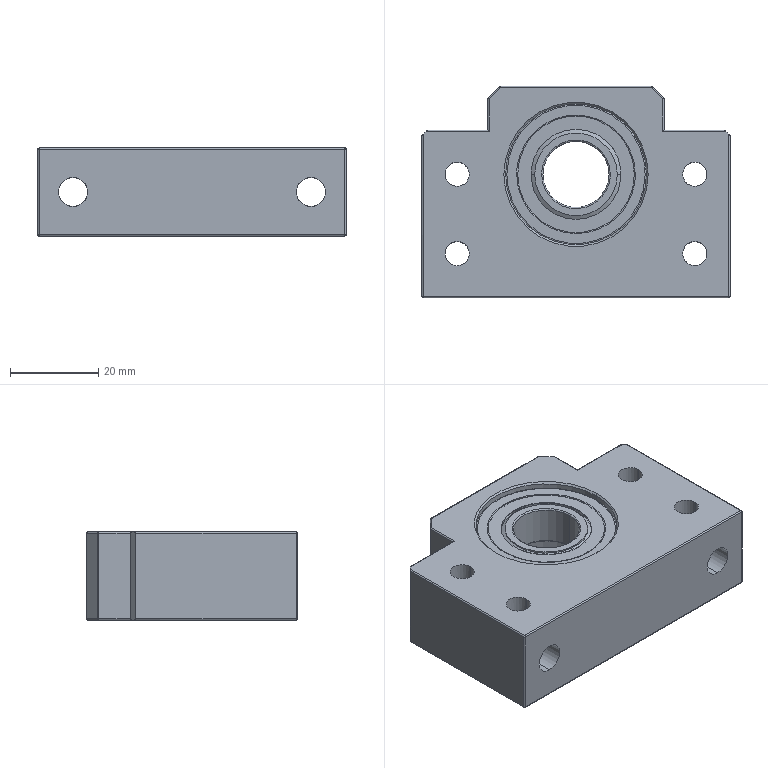Part | STEP file | 001-003-BF15 | 14 solids | 240 faces | box 70 x 48 x 20 mm | volume 44239 mm3 | cylinder 110 | spline 76 | plane 46 | cone 8 | commonest cylinder face diameters 0.528 x26 22.95 x21 24.05 x21 5.5 x16 6.6 x4 11 x4